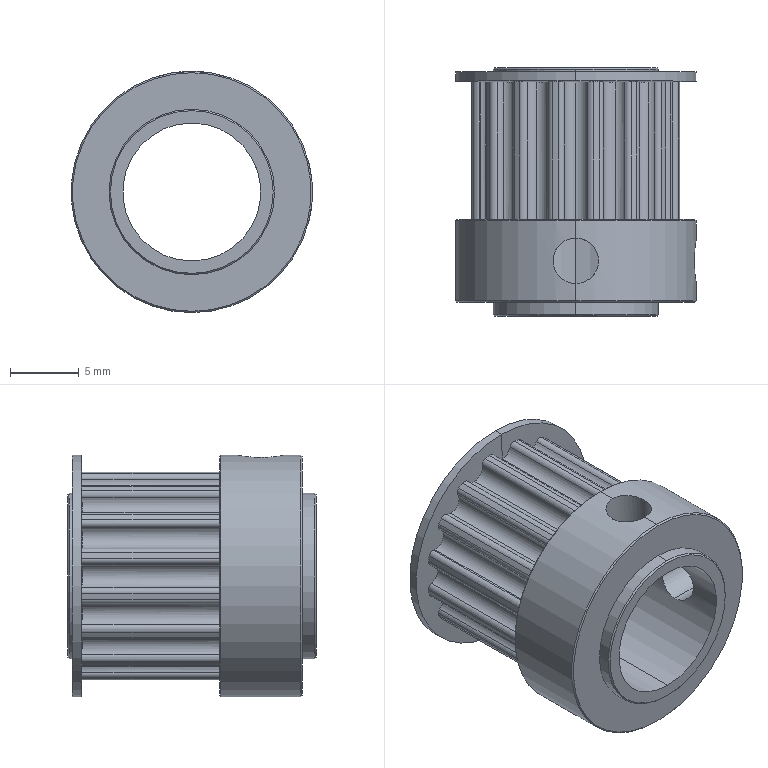Part | STEP file | Timing pulley 16-3M-Φ10-18 | 1 solid | 108 faces | box 17.5 x 18 x 17.5 mm | volume 1873 mm3 | cylinder 93 | cone 10 | plane 5 | commonest cylinder face diameters 0.8 x40 1.7 x23 15.28 x16 3.3 x4 12 x4 17.5 x4